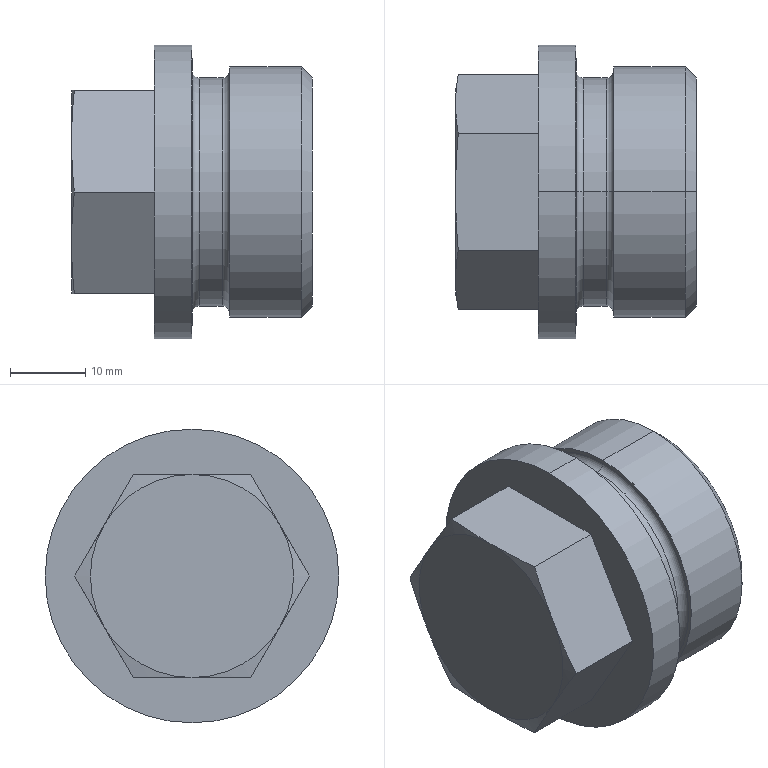Part | SolidWorks | features Boss 1, Cut 1, Fillet 1, Revolution 1 | 1 solid | 29 faces | box 32 x 39 x 39 mm | volume 25996 mm3 | plane 11 | cone 8 | cylinder 6 | torus 4 | commonest cylinder face diameters 30.291 x2 33.249 x2 39 x2
STEP:
#1=CARTESIAN_POINT('',(16.,0.,-16.145));
#2=VERTEX_POINT('',#1);
#3=CARTESIAN_POINT('',(16.,0.,16.145));
#4=VERTEX_POINT('',#3);
#5=CARTESIAN_POINT('',(16.,0.,0.));
#6=DIRECTION('',(-1.,0.,0.));
#7=DIRECTION('',(0.,0.,1.));
#8=AXIS2_PLACEMENT_3D('',#5,#6,#7);
#9=CIRCLE('',#8,16.145);
#10=EDGE_CURVE('',#2,#4,#9,.T.);
#11=ORIENTED_EDGE('',*,*,#10,.F.);
#12=CARTESIAN_POINT('',(17.,0.,-15.145));
#13=VERTEX_POINT('',#12);
#14=CARTESIAN_POINT('',(17.,0.,-16.145));
#15=DIRECTION('',(0.,1.,0.));
#16=DIRECTION('',(0.,0.,1.));
#17=AXIS2_PLACEMENT_3D('',#14,#15,#16);
#18=CIRCLE('',#17,1.);
#19=EDGE_CURVE('',#2,#13,#18,.T.);
#20=ORIENTED_EDGE('',*,*,#19,.T.);
#21=CARTESIAN_POINT('',(17.,0.,15.145));
#22=VERTEX_POINT('',#21);
#23=CARTESIAN_POINT('',(17.,0.,0.));
#24=DIRECTION('',(1.,0.,0.));
#25=DIRECTION('',(0.,0.,1.));
#26=AXIS2_PLACEMENT_3D('',#23,#24,#25);
#27=CIRCLE('',#26,15.145);
#28=EDGE_CURVE('',#22,#13,#27,.T.);
#29=ORIENTED_EDGE('',*,*,#28,.F.);
#30=CARTESIAN_POINT('',(17.,0.,16.145));
#31=DIRECTION('',(0.,-1.,0.));
#32=DIRECTION('',(0.,0.,-1.));
#33=AXIS2_PLACEMENT_3D('',#30,#31,#32);
#34=CIRCLE('',#33,1.);
#35=EDGE_CURVE('',#4,#22,#34,.T.);
#36=ORIENTED_EDGE('',*,*,#35,.F.);
#37=EDGE_LOOP('',(#11,#20,#29,#36));
#38=FACE_OUTER_BOUND('',#37,.T.);
#39=CARTESIAN_POINT('',(17.,0.,0.));
#40=DIRECTION('',(-1.,0.,0.));
#41=DIRECTION('',(0.,0.,1.));
#42=AXIS2_PLACEMENT_3D('',#39,#40,#41);
#43=TOROIDAL_SURFACE('',#42,16.145,1.);
#44=ADVANCED_FACE('',(#38),#43,.F.);
#45=CARTESIAN_POINT('',(21.,0.,16.145));
#46=VERTEX_POINT('',#45);
#47=CARTESIAN_POINT('',(21.,0.,-16.145));
#48=VERTEX_POINT('',#47);
#49=CARTESIAN_POINT('',(21.,0.,0.));
#50=DIRECTION('',(1.,0.,0.));
#51=DIRECTION('',(0.,0.,-1.));
#52=AXIS2_PLACEMENT_3D('',#49,#50,#51);
#53=CIRCLE('',#52,16.145);
#54=EDGE_CURVE('',#46,#48,#53,.T.);
#55=ORIENTED_EDGE('',*,*,#54,.F.);
#56=CARTESIAN_POINT('',(20.,0.,15.145));
#57=VERTEX_POINT('',#56);
#58=CARTESIAN_POINT('',(20.,0.,16.145));
#59=DIRECTION('',(0.,1.,0.));
#60=DIRECTION('',(0.,0.,1.));
#61=AXIS2_PLACEMENT_3D('',#58,#59,#60);
#62=CIRCLE('',#61,1.);
#63=EDGE_CURVE('',#46,#57,#62,.T.);
#64=ORIENTED_EDGE('',*,*,#63,.T.);
#65=CARTESIAN_POINT('',(20.,0.,-15.145));
#66=VERTEX_POINT('',#65);
#67=CARTESIAN_POINT('',(20.,0.,0.));
#68=DIRECTION('',(-1.,0.,0.));
#69=DIRECTION('',(0.,0.,-1.));
#70=AXIS2_PLACEMENT_3D('',#67,#68,#69);
#71=CIRCLE('',#70,15.145);
#72=EDGE_CURVE('',#66,#57,#71,.T.);
#73=ORIENTED_EDGE('',*,*,#72,.F.);
#74=CARTESIAN_POINT('',(20.,0.,-16.145));
#75=DIRECTION('',(0.,-1.,0.));
#76=DIRECTION('',(0.,0.,-1.));
#77=AXIS2_PLACEMENT_3D('',#74,#75,#76);
#78=CIRCLE('',#77,1.);
#79=EDGE_CURVE('',#48,#66,#78,.T.);
#80=ORIENTED_EDGE('',*,*,#79,.F.);
#81=EDGE_LOOP('',(#55,#64,#73,#80));
#82=FACE_OUTER_BOUND('',#81,.T.);
#83=CARTESIAN_POINT('',(20.,0.,0.));
#84=DIRECTION('',(1.,0.,0.));
#85=DIRECTION('',(0.,0.,-1.));
#86=AXIS2_PLACEMENT_3D('',#83,#84,#85);
#87=TOROIDAL_SURFACE('',#86,16.145,1.);
#88=ADVANCED_FACE('',(#82),#87,.F.);
#89=CARTESIAN_POINT('',(32.,0.,15.146));
#90=VERTEX_POINT('',#89);
#91=CARTESIAN_POINT('',(32.,0.,-15.146));
#92=VERTEX_POINT('',#91);
#93=CARTESIAN_POINT('',(32.,0.,0.));
#94=DIRECTION('',(-1.,0.,0.));
#95=DIRECTION('',(0.,0.,1.));
#96=AXIS2_PLACEMENT_3D('',#93,#94,#95);
#97=CIRCLE('',#96,15.146);
#98=EDGE_CURVE('',#90,#92,#97,.T.);
#99=ORIENTED_EDGE('',*,*,#98,.T.);
#100=CARTESIAN_POINT('',(30.521,0.,-16.625));
#101=VERTEX_POINT('',#100);
#102=CARTESIAN_POINT('',(32.,0.,-15.146));
#103=DIRECTION('',(-0.7071,0.,-0.7071));
#104=VECTOR('',#103,1000.);
#105=LINE('',#102,#104);
#106=EDGE_CURVE('',#92,#101,#105,.T.);
#107=ORIENTED_EDGE('',*,*,#106,.T.);
#108=CARTESIAN_POINT('',(30.521,0.,16.625));
#109=VERTEX_POINT('',#108);
#110=CARTESIAN_POINT('',(30.521,0.,0.));
#111=DIRECTION('',(-1.,0.,0.));
#112=DIRECTION('',(0.,0.,1.));
#113=AXIS2_PLACEMENT_3D('',#110,#111,#112);
#114=CIRCLE('',#113,16.625);
#115=EDGE_CURVE('',#109,#101,#114,.T.);
#116=ORIENTED_EDGE('',*,*,#115,.F.);
#117=CARTESIAN_POINT('',(32.,0.,15.146));
#118=DIRECTION('',(-0.7071,0.,0.7071));
#119=VECTOR('',#118,1000.);
#120=LINE('',#117,#119);
#121=EDGE_CURVE('',#90,#109,#120,.T.);
#122=ORIENTED_EDGE('',*,*,#121,.F.);
#123=EDGE_LOOP('',(#99,#107,#116,#122));
#124=FACE_OUTER_BOUND('',#123,.T.);
#125=CARTESIAN_POINT('',(32.,0.,0.));
#126=DIRECTION('',(-1.,0.,0.));
#127=DIRECTION('',(0.,0.,1.));
#128=AXIS2_PLACEMENT_3D('',#125,#126,#127);
#129=CONICAL_SURFACE('',#128,15.146,0.7854);
#130=ADVANCED_FACE('',(#124),#129,.T.);
#131=ORIENTED_EDGE('',*,*,#115,.T.);
#132=CARTESIAN_POINT('',(21.,0.,-16.625));
#133=VERTEX_POINT('',#132);
#134=CARTESIAN_POINT('',(0.,0.,-16.625));
#135=DIRECTION('',(-1.,0.,0.));
#136=VECTOR('',#135,1000.);
#137=LINE('',#134,#136);
#138=EDGE_CURVE('',#101,#133,#137,.T.);
#139=ORIENTED_EDGE('',*,*,#138,.T.);
#140=CARTESIAN_POINT('',(21.,0.,16.625));
#141=VERTEX_POINT('',#140);
#142=CARTESIAN_POINT('',(21.,0.,0.));
#143=DIRECTION('',(-1.,0.,0.));
#144=DIRECTION('',(0.,0.,1.));
#145=AXIS2_PLACEMENT_3D('',#142,#143,#144);
#146=CIRCLE('',#145,16.625);
#147=EDGE_CURVE('',#141,#133,#146,.T.);
#148=ORIENTED_EDGE('',*,*,#147,.F.);
#149=CARTESIAN_POINT('',(0.,0.,16.625));
#150=DIRECTION('',(-1.,0.,0.));
#151=VECTOR('',#150,1000.);
#152=LINE('',#149,#151);
#153=EDGE_CURVE('',#109,#141,#152,.T.);
#154=ORIENTED_EDGE('',*,*,#153,.F.);
#155=EDGE_LOOP('',(#131,#139,#148,#154));
#156=FACE_OUTER_BOUND('',#155,.T.);
#157=CARTESIAN_POINT('',(0.,0.,0.));
#158=DIRECTION('',(-1.,0.,0.));
#159=DIRECTION('',(0.,0.,1.));
#160=AXIS2_PLACEMENT_3D('',#157,#158,#159);
#161=CYLINDRICAL_SURFACE('',#160,16.625);
#162=ADVANCED_FACE('',(#156),#161,.T.);
#163=CARTESIAN_POINT('',(20.,0.,0.));
#164=DIRECTION('',(-1.,0.,0.));
#165=DIRECTION('',(0.,0.,-1.));
#166=AXIS2_PLACEMENT_3D('',#163,#164,#165);
#167=CIRCLE('',#166,15.145);
#168=EDGE_CURVE('',#57,#66,#167,.T.);
#169=ORIENTED_EDGE('',*,*,#168,.T.);
#170=CARTESIAN_POINT('',(0.,0.,-15.145));
#171=DIRECTION('',(-1.,0.,0.));
#172=VECTOR('',#171,1000.);
#173=LINE('',#170,#172);
#174=EDGE_CURVE('',#66,#13,#173,.T.);
#175=ORIENTED_EDGE('',*,*,#174,.T.);
#176=CARTESIAN_POINT('',(17.,0.,0.));
#177=DIRECTION('',(1.,0.,0.));
#178=DIRECTION('',(0.,0.,1.));
#179=AXIS2_PLACEMENT_3D('',#176,#177,#178);
#180=CIRCLE('',#179,15.145);
#181=EDGE_CURVE('',#13,#22,#180,.T.);
#182=ORIENTED_EDGE('',*,*,#181,.T.);
#183=CARTESIAN_POINT('',(0.,0.,15.145));
#184=DIRECTION('',(-1.,0.,0.));
#185=VECTOR('',#184,1000.);
#186=LINE('',#183,#185);
#187=EDGE_CURVE('',#57,#22,#186,.T.);
#188=ORIENTED_EDGE('',*,*,#187,.F.);
#189=EDGE_LOOP('',(#169,#175,#182,#188));
#190=FACE_OUTER_BOUND('',#189,.T.);
#191=CARTESIAN_POINT('',(0.,0.,0.));
#192=DIRECTION('',(-1.,0.,0.));
#193=DIRECTION('',(0.,0.,1.));
#194=AXIS2_PLACEMENT_3D('',#191,#192,#193);
#195=CYLINDRICAL_SURFACE('',#194,15.145);
#196=ADVANCED_FACE('',(#190),#195,.T.);
#197=CARTESIAN_POINT('',(16.,0.,19.5));
#198=VERTEX_POINT('',#197);
#199=CARTESIAN_POINT('',(16.,0.,-19.5));
#200=VERTEX_POINT('',#199);
#201=CARTESIAN_POINT('',(16.,0.,0.));
#202=DIRECTION('',(-1.,0.,0.));
#203=DIRECTION('',(0.,0.,1.));
#204=AXIS2_PLACEMENT_3D('',#201,#202,#203);
#205=CIRCLE('',#204,19.5);
#206=EDGE_CURVE('',#198,#200,#205,.T.);
#207=ORIENTED_EDGE('',*,*,#206,.T.);
#208=CARTESIAN_POINT('',(11.,0.,-19.5));
#209=VERTEX_POINT('',#208);
#210=CARTESIAN_POINT('',(0.,0.,-19.5));
#211=DIRECTION('',(-1.,0.,0.));
#212=VECTOR('',#211,1000.);
#213=LINE('',#210,#212);
#214=EDGE_CURVE('',#200,#209,#213,.T.);
#215=ORIENTED_EDGE('',*,*,#214,.T.);
#216=CARTESIAN_POINT('',(11.,0.,19.5));
#217=VERTEX_POINT('',#216);
#218=CARTESIAN_POINT('',(11.,0.,0.));
#219=DIRECTION('',(-1.,0.,0.));
#220=DIRECTION('',(0.,0.,1.));
#221=AXIS2_PLACEMENT_3D('',#218,#219,#220);
#222=CIRCLE('',#221,19.5);
#223=EDGE_CURVE('',#217,#209,#222,.T.);
#224=ORIENTED_EDGE('',*,*,#223,.F.);
#225=CARTESIAN_POINT('',(0.,0.,19.5));
#226=DIRECTION('',(-1.,0.,0.));
#227=VECTOR('',#226,1000.);
#228=LINE('',#225,#227);
#229=EDGE_CURVE('',#198,#217,#228,.T.);
#230=ORIENTED_EDGE('',*,*,#229,.F.);
#231=EDGE_LOOP('',(#207,#215,#224,#230));
#232=FACE_OUTER_BOUND('',#231,.T.);
#233=CARTESIAN_POINT('',(0.,0.,0.));
#234=DIRECTION('',(-1.,0.,0.));
#235=DIRECTION('',(0.,0.,1.));
#236=AXIS2_PLACEMENT_3D('',#233,#234,#235);
#237=CYLINDRICAL_SURFACE('',#236,19.5);
#238=ADVANCED_FACE('',(#232),#237,.T.);
#239=CARTESIAN_POINT('',(11.,7.794,-13.5));
#240=VERTEX_POINT('',#239);
#241=CARTESIAN_POINT('',(0.3683,7.794,-13.5));
#242=VERTEX_POINT('',#241);
#243=CARTESIAN_POINT('',(52.243,7.794,-13.5));
#244=DIRECTION('',(-1.,0.,0.));
#245=VECTOR('',#244,1000.);
#246=LINE('',#243,#245);
#247=EDGE_CURVE('',#240,#242,#246,.T.);
#248=ORIENTED_EDGE('',*,*,#247,.T.);
#249=CARTESIAN_POINT('',(0.,11.691,-6.75));
#250=VERTEX_POINT('',#249);
#251=CARTESIAN_POINT('',(0.3683,7.794,-13.5));
#252=CARTESIAN_POINT('',(0.2537,8.444,-12.375));
#253=CARTESIAN_POINT('',(0.1607,9.093,-11.25));
#254=CARTESIAN_POINT('',(0.03367,10.392,-9.));
#255=CARTESIAN_POINT('',(0.,11.042,-7.875));
#256=CARTESIAN_POINT('',(0.,11.691,-6.75));
#257=B_SPLINE_CURVE_WITH_KNOTS('',3,(#251,#252,#253,#254,#255,#256),.UNSPECIFIED.,.F.,.F.,(4,2,4),(0.000000231,0.003897,0.007794),.UNSPECIFIED.);
#258=EDGE_CURVE('',#242,#250,#257,.T.);
#259=ORIENTED_EDGE('',*,*,#258,.T.);
#260=CARTESIAN_POINT('',(0.3683,15.588,0.));
#261=VERTEX_POINT('',#260);
#262=CARTESIAN_POINT('',(0.,11.691,-6.75));
#263=CARTESIAN_POINT('',(0.,12.341,-5.625));
#264=CARTESIAN_POINT('',(0.03367,12.99,-4.5));
#265=CARTESIAN_POINT('',(0.1607,14.289,-2.25));
#266=CARTESIAN_POINT('',(0.2537,14.939,-1.125));
#267=CARTESIAN_POINT('',(0.3683,15.588,0.));
#268=B_SPLINE_CURVE_WITH_KNOTS('',3,(#262,#263,#264,#265,#266,#267),.UNSPECIFIED.,.F.,.F.,(4,2,4),(0.007794,0.01169,0.01559),.UNSPECIFIED.);
#269=EDGE_CURVE('',#250,#261,#268,.T.);
#270=ORIENTED_EDGE('',*,*,#269,.T.);
#271=CARTESIAN_POINT('',(11.,15.588,0.));
#272=VERTEX_POINT('',#271);
#273=CARTESIAN_POINT('',(52.243,15.588,0.));
#274=DIRECTION('',(-1.,0.,0.));
#275=VECTOR('',#274,1000.);
#276=LINE('',#273,#275);
#277=EDGE_CURVE('',#272,#261,#276,.T.);
#278=ORIENTED_EDGE('',*,*,#277,.F.);
#279=CARTESIAN_POINT('',(11.,15.588,0.));
#280=DIRECTION('',(0.,-0.5,-0.866));
#281=VECTOR('',#280,1000.);
#282=LINE('',#279,#281);
#283=EDGE_CURVE('',#272,#240,#282,.T.);
#284=ORIENTED_EDGE('',*,*,#283,.T.);
#285=EDGE_LOOP('',(#248,#259,#270,#278,#284));
#286=FACE_OUTER_BOUND('',#285,.T.);
#287=CARTESIAN_POINT('',(52.243,15.588,0.));
#288=DIRECTION('',(0.,0.866,-0.5));
#289=DIRECTION('',(0.,0.5,0.866));
#290=AXIS2_PLACEMENT_3D('',#287,#288,#289);
#291=PLANE('',#290);
#292=ADVANCED_FACE('',(#286),#291,.T.);
#293=CARTESIAN_POINT('',(11.,-7.794,-13.5));
#294=VERTEX_POINT('',#293);
#295=CARTESIAN_POINT('',(0.3683,-7.794,-13.5));
#296=VERTEX_POINT('',#295);
#297=CARTESIAN_POINT('',(52.243,-7.794,-13.5));
#298=DIRECTION('',(-1.,0.,0.));
#299=VECTOR('',#298,1000.);
#300=LINE('',#297,#299);
#301=EDGE_CURVE('',#294,#296,#300,.T.);
#302=ORIENTED_EDGE('',*,*,#301,.T.);
#303=CARTESIAN_POINT('',(0.,0.,-13.5));
#304=VERTEX_POINT('',#303);
#305=CARTESIAN_POINT('',(0.3683,-7.794,-13.5));
#306=CARTESIAN_POINT('',(0.2539,-6.497,-13.5));
#307=CARTESIAN_POINT('',(0.1607,-5.196,-13.5));
#308=CARTESIAN_POINT('',(0.03364,-2.597,-13.5));
#309=CARTESIAN_POINT('',(0.,-1.298,-13.5));
#310=CARTESIAN_POINT('',(0.,0.,-13.5));
#311=B_SPLINE_CURVE_WITH_KNOTS('',3,(#305,#306,#307,#308,#309,#310),.UNSPECIFIED.,.F.,.F.,(4,2,4),(0.01311,0.01702,0.02092),.UNSPECIFIED.);
#312=EDGE_CURVE('',#296,#304,#311,.T.);
#313=ORIENTED_EDGE('',*,*,#312,.T.);
#314=CARTESIAN_POINT('',(0.,0.,-13.5));
#315=CARTESIAN_POINT('',(0.,1.3,-13.5));
#316=CARTESIAN_POINT('',(0.03372,2.6,-13.5));
#317=CARTESIAN_POINT('',(0.1608,5.198,-13.5));
#318=CARTESIAN_POINT('',(0.2538,6.496,-13.5));
#319=CARTESIAN_POINT('',(0.3683,7.794,-13.5));
#320=B_SPLINE_CURVE_WITH_KNOTS('',3,(#314,#315,#316,#317,#318,#319),.UNSPECIFIED.,.F.,.F.,(4,2,4),(0.02092,0.02483,0.02874),.UNSPECIFIED.);
#321=EDGE_CURVE('',#304,#242,#320,.T.);
#322=ORIENTED_EDGE('',*,*,#321,.T.);
#323=ORIENTED_EDGE('',*,*,#247,.F.);
#324=CARTESIAN_POINT('',(11.,7.794,-13.5));
#325=DIRECTION('',(0.,-1.,0.));
#326=VECTOR('',#325,1000.);
#327=LINE('',#324,#326);
#328=EDGE_CURVE('',#240,#294,#327,.T.);
#329=ORIENTED_EDGE('',*,*,#328,.T.);
#330=EDGE_LOOP('',(#302,#313,#322,#323,#329));
#331=FACE_OUTER_BOUND('',#330,.T.);
#332=CARTESIAN_POINT('',(52.243,7.794,-13.5));
#333=DIRECTION('',(0.,0.,-1.));
#334=DIRECTION('',(-1.,0.,0.));
#335=AXIS2_PLACEMENT_3D('',#332,#333,#334);
#336=PLANE('',#335);
#337=ADVANCED_FACE('',(#331),#336,.T.);
#338=CARTESIAN_POINT('',(11.,-15.588,0.));
#339=VERTEX_POINT('',#338);
#340=CARTESIAN_POINT('',(0.3683,-15.588,0.));
#341=VERTEX_POINT('',#340);
#342=CARTESIAN_POINT('',(52.243,-15.588,0.));
#343=DIRECTION('',(-1.,0.,0.));
#344=VECTOR('',#343,1000.);
#345=LINE('',#342,#344);
#346=EDGE_CURVE('',#339,#341,#345,.T.);
#347=ORIENTED_EDGE('',*,*,#346,.T.);
#348=CARTESIAN_POINT('',(0.,-11.691,-6.75));
#349=VERTEX_POINT('',#348);
#350=CARTESIAN_POINT('',(0.3683,-15.588,0.));
#351=CARTESIAN_POINT('',(0.2537,-14.939,-1.125));
#352=CARTESIAN_POINT('',(0.1607,-14.289,-2.25));
#353=CARTESIAN_POINT('',(0.03367,-12.99,-4.5));
#354=CARTESIAN_POINT('',(0.,-12.341,-5.625));
#355=CARTESIAN_POINT('',(0.,-11.691,-6.75));
#356=B_SPLINE_CURVE_WITH_KNOTS('',3,(#350,#351,#352,#353,#354,#355),.UNSPECIFIED.,.F.,.F.,(4,2,4),(0.000000231,0.003897,0.007794),.UNSPECIFIED.);
#357=EDGE_CURVE('',#341,#349,#356,.T.);
#358=ORIENTED_EDGE('',*,*,#357,.T.);
#359=CARTESIAN_POINT('',(0.,-11.691,-6.75));
#360=CARTESIAN_POINT('',(0.,-11.042,-7.875));
#361=CARTESIAN_POINT('',(0.03367,-10.392,-9.));
#362=CARTESIAN_POINT('',(0.1607,-9.093,-11.25));
#363=CARTESIAN_POINT('',(0.2537,-8.444,-12.375));
#364=CARTESIAN_POINT('',(0.3683,-7.794,-13.5));
#365=B_SPLINE_CURVE_WITH_KNOTS('',3,(#359,#360,#361,#362,#363,#364),.UNSPECIFIED.,.F.,.F.,(4,2,4),(0.007794,0.01169,0.01559),.UNSPECIFIED.);
#366=EDGE_CURVE('',#349,#296,#365,.T.);
#367=ORIENTED_EDGE('',*,*,#366,.T.);
#368=ORIENTED_EDGE('',*,*,#301,.F.);
#369=CARTESIAN_POINT('',(11.,-7.794,-13.5));
#370=DIRECTION('',(0.,-0.5,0.866));
#371=VECTOR('',#370,1000.);
#372=LINE('',#369,#371);
#373=EDGE_CURVE('',#294,#339,#372,.T.);
#374=ORIENTED_EDGE('',*,*,#373,.T.);
#375=EDGE_LOOP('',(#347,#358,#367,#368,#374));
#376=FACE_OUTER_BOUND('',#375,.T.);
#377=CARTESIAN_POINT('',(52.243,-7.794,-13.5));
#378=DIRECTION('',(0.,-0.866,-0.5));
#379=DIRECTION('',(0.,0.5,-0.866));
#380=AXIS2_PLACEMENT_3D('',#377,#378,#379);
#381=PLANE('',#380);
#382=ADVANCED_FACE('',(#376),#381,.T.);
#383=CARTESIAN_POINT('',(11.,-7.794,13.5));
#384=VERTEX_POINT('',#383);
#385=CARTESIAN_POINT('',(0.3683,-7.794,13.5));
#386=VERTEX_POINT('',#385);
#387=CARTESIAN_POINT('',(52.243,-7.794,13.5));
#388=DIRECTION('',(-1.,0.,0.));
#389=VECTOR('',#388,1000.);
#390=LINE('',#387,#389);
#391=EDGE_CURVE('',#384,#386,#390,.T.);
#392=ORIENTED_EDGE('',*,*,#391,.T.);
#393=CARTESIAN_POINT('',(0.,-11.691,6.75));
#394=VERTEX_POINT('',#393);
#395=CARTESIAN_POINT('',(0.3683,-7.794,13.5));
#396=CARTESIAN_POINT('',(0.2537,-8.444,12.375));
#397=CARTESIAN_POINT('',(0.1607,-9.093,11.25));
#398=CARTESIAN_POINT('',(0.03367,-10.392,9.));
#399=CARTESIAN_POINT('',(0.,-11.042,7.875));
#400=CARTESIAN_POINT('',(0.,-11.691,6.75));
#401=B_SPLINE_CURVE_WITH_KNOTS('',3,(#395,#396,#397,#398,#399,#400),.UNSPECIFIED.,.F.,.F.,(4,2,4),(0.000000231,0.003897,0.007794),.UNSPECIFIED.);
#402=EDGE_CURVE('',#386,#394,#401,.T.);
#403=ORIENTED_EDGE('',*,*,#402,.T.);
#404=CARTESIAN_POINT('',(0.,-11.691,6.75));
#405=CARTESIAN_POINT('',(0.,-12.341,5.625));
#406=CARTESIAN_POINT('',(0.03367,-12.99,4.5));
#407=CARTESIAN_POINT('',(0.1607,-14.289,2.25));
#408=CARTESIAN_POINT('',(0.2537,-14.939,1.125));
#409=CARTESIAN_POINT('',(0.3683,-15.588,0.));
#410=B_SPLINE_CURVE_WITH_KNOTS('',3,(#404,#405,#406,#407,#408,#409),.UNSPECIFIED.,.F.,.F.,(4,2,4),(0.007794,0.01169,0.01559),.UNSPECIFIED.);
#411=EDGE_CURVE('',#394,#341,#410,.T.);
#412=ORIENTED_EDGE('',*,*,#411,.T.);
#413=ORIENTED_EDGE('',*,*,#346,.F.);
#414=CARTESIAN_POINT('',(11.,-15.588,0.));
#415=DIRECTION('',(0.,0.5,0.866));
#416=VECTOR('',#415,1000.);
#417=LINE('',#414,#416);
#418=EDGE_CURVE('',#339,#384,#417,.T.);
#419=ORIENTED_EDGE('',*,*,#418,.T.);
#420=EDGE_LOOP('',(#392,#403,#412,#413,#419));
#421=FACE_OUTER_BOUND('',#420,.T.);
#422=CARTESIAN_POINT('',(52.243,-15.588,0.));
#423=DIRECTION('',(0.,-0.866,0.5));
#424=DIRECTION('',(0.,-0.5,-0.866));
#425=AXIS2_PLACEMENT_3D('',#422,#423,#424);
#426=PLANE('',#425);
#427=ADVANCED_FACE('',(#421),#426,.T.);
#428=CARTESIAN_POINT('',(11.,7.794,13.5));
#429=VERTEX_POINT('',#428);
#430=CARTESIAN_POINT('',(0.3683,7.794,13.5));
#431=VERTEX_POINT('',#430);
#432=CARTESIAN_POINT('',(52.243,7.794,13.5));
#433=DIRECTION('',(-1.,0.,0.));
#434=VECTOR('',#433,1000.);
#435=LINE('',#432,#434);
#436=EDGE_CURVE('',#429,#431,#435,.T.);
#437=ORIENTED_EDGE('',*,*,#436,.T.);
#438=CARTESIAN_POINT('',(0.,0.,13.5));
#439=VERTEX_POINT('',#438);
#440=CARTESIAN_POINT('',(0.3683,7.794,13.5));
#441=CARTESIAN_POINT('',(0.2538,6.496,13.5));
#442=CARTESIAN_POINT('',(0.1608,5.198,13.5));
#443=CARTESIAN_POINT('',(0.03372,2.6,13.5));
#444=CARTESIAN_POINT('',(0.,1.3,13.5));
#445=CARTESIAN_POINT('',(0.,0.,13.5));
#446=B_SPLINE_CURVE_WITH_KNOTS('',3,(#440,#441,#442,#443,#444,#445),.UNSPECIFIED.,.F.,.F.,(4,2,4),(0.03715,0.04105,0.04496),.UNSPECIFIED.);
#447=EDGE_CURVE('',#431,#439,#446,.T.);
#448=ORIENTED_EDGE('',*,*,#447,.T.);
#449=CARTESIAN_POINT('',(0.,0.,13.5));
#450=CARTESIAN_POINT('',(0.,-1.298,13.5));
#451=CARTESIAN_POINT('',(0.03364,-2.597,13.5));
#452=CARTESIAN_POINT('',(0.1607,-5.196,13.5));
#453=CARTESIAN_POINT('',(0.2539,-6.497,13.5));
#454=CARTESIAN_POINT('',(0.3683,-7.794,13.5));
#455=B_SPLINE_CURVE_WITH_KNOTS('',3,(#449,#450,#451,#452,#453,#454),.UNSPECIFIED.,.F.,.F.,(4,2,4),(0.04496,0.04886,0.05276),.UNSPECIFIED.);
#456=EDGE_CURVE('',#439,#386,#455,.T.);
#457=ORIENTED_EDGE('',*,*,#456,.T.);
#458=ORIENTED_EDGE('',*,*,#391,.F.);
#459=CARTESIAN_POINT('',(11.,-7.794,13.5));
#460=DIRECTION('',(0.,1.,0.));
#461=VECTOR('',#460,1000.);
#462=LINE('',#459,#461);
#463=EDGE_CURVE('',#384,#429,#462,.T.);
#464=ORIENTED_EDGE('',*,*,#463,.T.);
#465=EDGE_LOOP('',(#437,#448,#457,#458,#464));
#466=FACE_OUTER_BOUND('',#465,.T.);
#467=CARTESIAN_POINT('',(52.243,-7.794,13.5));
#468=DIRECTION('',(0.,0.,1.));
#469=DIRECTION('',(0.,-1.,0.));
#470=AXIS2_PLACEMENT_3D('',#467,#468,#469);
#471=PLANE('',#470);
#472=ADVANCED_FACE('',(#466),#471,.T.);
#473=ORIENTED_EDGE('',*,*,#277,.T.);
#474=CARTESIAN_POINT('',(0.,11.691,6.75));
#475=VERTEX_POINT('',#474);
#476=CARTESIAN_POINT('',(0.3683,15.588,0.));
#477=CARTESIAN_POINT('',(0.2537,14.939,1.125));
#478=CARTESIAN_POINT('',(0.1607,14.289,2.25));
#479=CARTESIAN_POINT('',(0.03367,12.99,4.5));
#480=CARTESIAN_POINT('',(0.,12.341,5.625));
#481=CARTESIAN_POINT('',(0.,11.691,6.75));
#482=B_SPLINE_CURVE_WITH_KNOTS('',3,(#476,#477,#478,#479,#480,#481),.UNSPECIFIED.,.F.,.F.,(4,2,4),(0.000000231,0.003897,0.007794),.UNSPECIFIED.);
#483=EDGE_CURVE('',#261,#475,#482,.T.);
#484=ORIENTED_EDGE('',*,*,#483,.T.);
#485=CARTESIAN_POINT('',(0.,11.691,6.75));
#486=CARTESIAN_POINT('',(0.,11.042,7.875));
#487=CARTESIAN_POINT('',(0.03367,10.392,9.));
#488=CARTESIAN_POINT('',(0.1607,9.093,11.25));
#489=CARTESIAN_POINT('',(0.2537,8.444,12.375));
#490=CARTESIAN_POINT('',(0.3683,7.794,13.5));
#491=B_SPLINE_CURVE_WITH_KNOTS('',3,(#485,#486,#487,#488,#489,#490),.UNSPECIFIED.,.F.,.F.,(4,2,4),(0.007794,0.01169,0.01559),.UNSPECIFIED.);
#492=EDGE_CURVE('',#475,#431,#491,.T.);
#493=ORIENTED_EDGE('',*,*,#492,.T.);
#494=ORIENTED_EDGE('',*,*,#436,.F.);
#495=CARTESIAN_POINT('',(11.,7.794,13.5));
#496=DIRECTION('',(0.,0.5,-0.866));
#497=VECTOR('',#496,1000.);
#498=LINE('',#495,#497);
#499=EDGE_CURVE('',#429,#272,#498,.T.);
#500=ORIENTED_EDGE('',*,*,#499,.T.);
#501=EDGE_LOOP('',(#473,#484,#493,#494,#500));
#502=FACE_OUTER_BOUND('',#501,.T.);
#503=CARTESIAN_POINT('',(52.243,7.794,13.5));
#504=DIRECTION('',(0.,0.866,0.5));
#505=DIRECTION('',(0.,-0.5,0.866));
#506=AXIS2_PLACEMENT_3D('',#503,#504,#505);
#507=PLANE('',#506);
#508=ADVANCED_FACE('',(#502),#507,.T.);
#509=ORIENTED_EDGE('',*,*,#328,.F.);
#510=ORIENTED_EDGE('',*,*,#283,.F.);
#511=ORIENTED_EDGE('',*,*,#499,.F.);
#512=ORIENTED_EDGE('',*,*,#463,.F.);
#513=ORIENTED_EDGE('',*,*,#418,.F.);
#514=ORIENTED_EDGE('',*,*,#373,.F.);
#515=EDGE_LOOP('',(#509,#510,#511,#512,#513,#514));
#516=FACE_BOUND('',#515,.T.);
#517=ORIENTED_EDGE('',*,*,#223,.T.);
#518=CARTESIAN_POINT('',(11.,0.,0.));
#519=DIRECTION('',(-1.,0.,0.));
#520=DIRECTION('',(0.,0.,1.));
#521=AXIS2_PLACEMENT_3D('',#518,#519,#520);
#522=CIRCLE('',#521,19.5);
#523=EDGE_CURVE('',#209,#217,#522,.T.);
#524=ORIENTED_EDGE('',*,*,#523,.T.);
#525=EDGE_LOOP('',(#517,#524));
#526=FACE_OUTER_BOUND('',#525,.T.);
#527=CARTESIAN_POINT('',(11.,19.5,0.));
#528=DIRECTION('',(1.,0.,0.));
#529=DIRECTION('',(0.,0.,-1.));
#530=AXIS2_PLACEMENT_3D('',#527,#528,#529);
#531=PLANE('',#530);
#532=ADVANCED_FACE('',(#516,#526),#531,.F.);
#533=ORIENTED_EDGE('',*,*,#214,.F.);
#534=CARTESIAN_POINT('',(16.,0.,0.));
#535=DIRECTION('',(-1.,0.,0.));
#536=DIRECTION('',(0.,0.,1.));
#537=AXIS2_PLACEMENT_3D('',#534,#535,#536);
#538=CIRCLE('',#537,19.5);
#539=EDGE_CURVE('',#200,#198,#538,.T.);
#540=ORIENTED_EDGE('',*,*,#539,.T.);
#541=ORIENTED_EDGE('',*,*,#229,.T.);
#542=ORIENTED_EDGE('',*,*,#523,.F.);
#543=EDGE_LOOP('',(#533,#540,#541,#542));
#544=FACE_OUTER_BOUND('',#543,.T.);
#545=CARTESIAN_POINT('',(0.,0.,0.));
#546=DIRECTION('',(-1.,0.,0.));
#547=DIRECTION('',(0.,0.,1.));
#548=AXIS2_PLACEMENT_3D('',#545,#546,#547);
#549=CYLINDRICAL_SURFACE('',#548,19.5);
#550=ADVANCED_FACE('',(#544),#549,.T.);
#551=CARTESIAN_POINT('',(16.,0.,0.));
#552=DIRECTION('',(-1.,0.,0.));
#553=DIRECTION('',(0.,0.,1.));
#554=AXIS2_PLACEMENT_3D('',#551,#552,#553);
#555=CIRCLE('',#554,16.145);
#556=EDGE_CURVE('',#4,#2,#555,.T.);
#557=ORIENTED_EDGE('',*,*,#556,.T.);
#558=ORIENTED_EDGE('',*,*,#10,.T.);
#559=EDGE_LOOP('',(#557,#558));
#560=FACE_BOUND('',#559,.T.);
#561=ORIENTED_EDGE('',*,*,#206,.F.);
#562=ORIENTED_EDGE('',*,*,#539,.F.);
#563=EDGE_LOOP('',(#561,#562));
#564=FACE_OUTER_BOUND('',#563,.T.);
#565=CARTESIAN_POINT('',(16.,15.145,0.));
#566=DIRECTION('',(-1.,0.,0.));
#567=DIRECTION('',(0.,0.,1.));
#568=AXIS2_PLACEMENT_3D('',#565,#566,#567);
#569=PLANE('',#568);
#570=ADVANCED_FACE('',(#560,#564),#569,.F.);
#571=ORIENTED_EDGE('',*,*,#174,.F.);
#572=ORIENTED_EDGE('',*,*,#72,.T.);
#573=ORIENTED_EDGE('',*,*,#187,.T.);
#574=ORIENTED_EDGE('',*,*,#28,.T.);
#575=EDGE_LOOP('',(#571,#572,#573,#574));
#576=FACE_OUTER_BOUND('',#575,.T.);
#577=CARTESIAN_POINT('',(0.,0.,0.));
#578=DIRECTION('',(-1.,0.,0.));
#579=DIRECTION('',(0.,0.,1.));
#580=AXIS2_PLACEMENT_3D('',#577,#578,#579);
#581=CYLINDRICAL_SURFACE('',#580,15.145);
#582=ADVANCED_FACE('',(#576),#581,.T.);
#583=CARTESIAN_POINT('',(21.,0.,0.));
#584=DIRECTION('',(1.,0.,0.));
#585=DIRECTION('',(0.,0.,-1.));
#586=AXIS2_PLACEMENT_3D('',#583,#584,#585);
#587=CIRCLE('',#586,16.145);
#588=EDGE_CURVE('',#48,#46,#587,.T.);
#589=ORIENTED_EDGE('',*,*,#588,.T.);
#590=ORIENTED_EDGE('',*,*,#54,.T.);
#591=EDGE_LOOP('',(#589,#590));
#592=FACE_BOUND('',#591,.T.);
#593=ORIENTED_EDGE('',*,*,#147,.T.);
#594=CARTESIAN_POINT('',(21.,0.,0.));
#595=DIRECTION('',(-1.,0.,0.));
#596=DIRECTION('',(0.,0.,1.));
#597=AXIS2_PLACEMENT_3D('',#594,#595,#596);
#598=CIRCLE('',#597,16.625);
#599=EDGE_CURVE('',#133,#141,#598,.T.);
#600=ORIENTED_EDGE('',*,*,#599,.T.);
#601=EDGE_LOOP('',(#593,#600));
#602=FACE_OUTER_BOUND('',#601,.T.);
#603=CARTESIAN_POINT('',(21.,16.625,0.));
#604=DIRECTION('',(1.,0.,0.));
#605=DIRECTION('',(0.,0.,-1.));
#606=AXIS2_PLACEMENT_3D('',#603,#604,#605);
#607=PLANE('',#606);
#608=ADVANCED_FACE('',(#592,#602),#607,.F.);
#609=ORIENTED_EDGE('',*,*,#138,.F.);
#610=CARTESIAN_POINT('',(30.521,0.,0.));
#611=DIRECTION('',(-1.,0.,0.));
#612=DIRECTION('',(0.,0.,1.));
#613=AXIS2_PLACEMENT_3D('',#610,#611,#612);
#614=CIRCLE('',#613,16.625);
#615=EDGE_CURVE('',#101,#109,#614,.T.);
#616=ORIENTED_EDGE('',*,*,#615,.T.);
#617=ORIENTED_EDGE('',*,*,#153,.T.);
#618=ORIENTED_EDGE('',*,*,#599,.F.);
#619=EDGE_LOOP('',(#609,#616,#617,#618));
#620=FACE_OUTER_BOUND('',#619,.T.);
#621=CARTESIAN_POINT('',(0.,0.,0.));
#622=DIRECTION('',(-1.,0.,0.));
#623=DIRECTION('',(0.,0.,1.));
#624=AXIS2_PLACEMENT_3D('',#621,#622,#623);
#625=CYLINDRICAL_SURFACE('',#624,16.625);
#626=ADVANCED_FACE('',(#620),#625,.T.);
#627=ORIENTED_EDGE('',*,*,#106,.F.);
#628=CARTESIAN_POINT('',(32.,0.,0.));
#629=DIRECTION('',(-1.,0.,0.));
#630=DIRECTION('',(0.,0.,1.));
#631=AXIS2_PLACEMENT_3D('',#628,#629,#630);
#632=CIRCLE('',#631,15.146);
#633=EDGE_CURVE('',#92,#90,#632,.T.);
#634=ORIENTED_EDGE('',*,*,#633,.T.);
#635=ORIENTED_EDGE('',*,*,#121,.T.);
#636=ORIENTED_EDGE('',*,*,#615,.F.);
#637=EDGE_LOOP('',(#627,#634,#635,#636));
#638=FACE_OUTER_BOUND('',#637,.T.);
#639=CARTESIAN_POINT('',(32.,0.,0.));
#640=DIRECTION('',(-1.,0.,0.));
#641=DIRECTION('',(0.,0.,1.));
#642=AXIS2_PLACEMENT_3D('',#639,#640,#641);
#643=CONICAL_SURFACE('',#642,15.146,0.7854);
#644=ADVANCED_FACE('',(#638),#643,.T.);
#645=ORIENTED_EDGE('',*,*,#98,.F.);
#646=ORIENTED_EDGE('',*,*,#633,.F.);
#647=EDGE_LOOP('',(#645,#646));
#648=FACE_OUTER_BOUND('',#647,.T.);
#649=CARTESIAN_POINT('',(32.,15.146,0.));
#650=DIRECTION('',(-1.,0.,0.));
#651=DIRECTION('',(0.,0.,1.));
#652=AXIS2_PLACEMENT_3D('',#649,#650,#651);
#653=PLANE('',#652);
#654=ADVANCED_FACE('',(#648),#653,.F.);
#655=CARTESIAN_POINT('',(0.,0.,0.));
#656=DIRECTION('',(1.,0.,0.));
#657=DIRECTION('',(0.,0.,-1.));
#658=AXIS2_PLACEMENT_3D('',#655,#656,#657);
#659=CIRCLE('',#658,13.5);
#660=EDGE_CURVE('',#349,#304,#659,.T.);
#661=ORIENTED_EDGE('',*,*,#660,.T.);
#662=ORIENTED_EDGE('',*,*,#312,.F.);
#663=ORIENTED_EDGE('',*,*,#366,.F.);
#664=EDGE_LOOP('',(#661,#662,#663));
#665=FACE_OUTER_BOUND('',#664,.T.);
#666=CARTESIAN_POINT('',(0.,0.,0.));
#667=DIRECTION('',(1.,0.,0.));
#668=DIRECTION('',(0.,0.,1.));
#669=AXIS2_PLACEMENT_3D('',#666,#667,#668);
#670=CONICAL_SURFACE('',#669,13.5,1.396);
#671=ADVANCED_FACE('',(#665),#670,.T.);
#672=ORIENTED_EDGE('',*,*,#411,.F.);
#673=CARTESIAN_POINT('',(0.,0.,0.));
#674=DIRECTION('',(1.,0.,0.));
#675=DIRECTION('',(0.,0.,-1.));
#676=AXIS2_PLACEMENT_3D('',#673,#674,#675);
#677=CIRCLE('',#676,13.5);
#678=EDGE_CURVE('',#394,#349,#677,.T.);
#679=ORIENTED_EDGE('',*,*,#678,.T.);
#680=ORIENTED_EDGE('',*,*,#357,.F.);
#681=EDGE_LOOP('',(#672,#679,#680));
#682=FACE_OUTER_BOUND('',#681,.T.);
#683=CARTESIAN_POINT('',(0.,0.,0.));
#684=DIRECTION('',(1.,0.,0.));
#685=DIRECTION('',(0.,0.,1.));
#686=AXIS2_PLACEMENT_3D('',#683,#684,#685);
#687=CONICAL_SURFACE('',#686,13.5,1.396);
#688=ADVANCED_FACE('',(#682),#687,.T.);
#689=ORIENTED_EDGE('',*,*,#456,.F.);
#690=CARTESIAN_POINT('',(0.,0.,0.));
#691=DIRECTION('',(1.,0.,0.));
#692=DIRECTION('',(0.,0.,-1.));
#693=AXIS2_PLACEMENT_3D('',#690,#691,#692);
#694=CIRCLE('',#693,13.5);
#695=EDGE_CURVE('',#439,#394,#694,.T.);
#696=ORIENTED_EDGE('',*,*,#695,.T.);
#697=ORIENTED_EDGE('',*,*,#402,.F.);
#698=EDGE_LOOP('',(#689,#696,#697));
#699=FACE_OUTER_BOUND('',#698,.T.);
#700=CARTESIAN_POINT('',(0.,0.,0.));
#701=DIRECTION('',(1.,0.,0.));
#702=DIRECTION('',(0.,0.,1.));
#703=AXIS2_PLACEMENT_3D('',#700,#701,#702);
#704=CONICAL_SURFACE('',#703,13.5,1.396);
#705=ADVANCED_FACE('',(#699),#704,.T.);
#706=ORIENTED_EDGE('',*,*,#492,.F.);
#707=CARTESIAN_POINT('',(0.,0.,0.));
#708=DIRECTION('',(-1.,0.,0.));
#709=DIRECTION('',(0.,0.,1.));
#710=AXIS2_PLACEMENT_3D('',#707,#708,#709);
#711=CIRCLE('',#710,13.5);
#712=EDGE_CURVE('',#439,#475,#711,.T.);
#713=ORIENTED_EDGE('',*,*,#712,.F.);
#714=ORIENTED_EDGE('',*,*,#447,.F.);
#715=EDGE_LOOP('',(#706,#713,#714));
#716=FACE_OUTER_BOUND('',#715,.T.);
#717=CARTESIAN_POINT('',(0.,0.,0.));
#718=DIRECTION('',(1.,0.,0.));
#719=DIRECTION('',(0.,0.,1.));
#720=AXIS2_PLACEMENT_3D('',#717,#718,#719);
#721=CONICAL_SURFACE('',#720,13.5,1.396);
#722=ADVANCED_FACE('',(#716),#721,.T.);
#723=CARTESIAN_POINT('',(0.,0.,0.));
#724=DIRECTION('',(1.,0.,0.));
#725=DIRECTION('',(0.,0.,-1.));
#726=AXIS2_PLACEMENT_3D('',#723,#724,#725);
#727=CIRCLE('',#726,13.5);
#728=EDGE_CURVE('',#250,#475,#727,.T.);
#729=ORIENTED_EDGE('',*,*,#728,.T.);
#730=ORIENTED_EDGE('',*,*,#483,.F.);
#731=ORIENTED_EDGE('',*,*,#269,.F.);
#732=EDGE_LOOP('',(#729,#730,#731));
#733=FACE_OUTER_BOUND('',#732,.T.);
#734=CARTESIAN_POINT('',(0.,0.,0.));
#735=DIRECTION('',(1.,0.,0.));
#736=DIRECTION('',(0.,0.,1.));
#737=AXIS2_PLACEMENT_3D('',#734,#735,#736);
#738=CONICAL_SURFACE('',#737,13.5,1.396);
#739=ADVANCED_FACE('',(#733),#738,.T.);
#740=CARTESIAN_POINT('',(0.,0.,0.));
#741=DIRECTION('',(1.,0.,0.));
#742=DIRECTION('',(0.,0.,-1.));
#743=AXIS2_PLACEMENT_3D('',#740,#741,#742);
#744=CIRCLE('',#743,13.5);
#745=EDGE_CURVE('',#304,#250,#744,.T.);
#746=ORIENTED_EDGE('',*,*,#745,.T.);
#747=ORIENTED_EDGE('',*,*,#258,.F.);
#748=ORIENTED_EDGE('',*,*,#321,.F.);
#749=EDGE_LOOP('',(#746,#747,#748));
#750=FACE_OUTER_BOUND('',#749,.T.);
#751=CARTESIAN_POINT('',(0.,0.,0.));
#752=DIRECTION('',(1.,0.,0.));
#753=DIRECTION('',(0.,0.,1.));
#754=AXIS2_PLACEMENT_3D('',#751,#752,#753);
#755=CONICAL_SURFACE('',#754,13.5,1.396);
#756=ADVANCED_FACE('',(#750),#755,.T.);
#757=ORIENTED_EDGE('',*,*,#745,.F.);
#758=ORIENTED_EDGE('',*,*,#660,.F.);
#759=ORIENTED_EDGE('',*,*,#678,.F.);
#760=ORIENTED_EDGE('',*,*,#695,.F.);
#761=ORIENTED_EDGE('',*,*,#712,.T.);
#762=ORIENTED_EDGE('',*,*,#728,.F.);
#763=EDGE_LOOP('',(#757,#758,#759,#760,#761,#762));
#764=FACE_OUTER_BOUND('',#763,.T.);
#765=CARTESIAN_POINT('',(0.,1.5,0.));
#766=DIRECTION('',(1.,0.,0.));
#767=DIRECTION('',(0.,0.,-1.));
#768=AXIS2_PLACEMENT_3D('',#765,#766,#767);
#769=PLANE('',#768);
#770=ADVANCED_FACE('',(#764),#769,.F.);
#771=ORIENTED_EDGE('',*,*,#63,.F.);
#772=ORIENTED_EDGE('',*,*,#588,.F.);
#773=ORIENTED_EDGE('',*,*,#79,.T.);
#774=ORIENTED_EDGE('',*,*,#168,.F.);
#775=EDGE_LOOP('',(#771,#772,#773,#774));
#776=FACE_OUTER_BOUND('',#775,.T.);
#777=CARTESIAN_POINT('',(20.,0.,0.));
#778=DIRECTION('',(1.,0.,0.));
#779=DIRECTION('',(0.,0.,-1.));
#780=AXIS2_PLACEMENT_3D('',#777,#778,#779);
#781=TOROIDAL_SURFACE('',#780,16.145,1.);
#782=ADVANCED_FACE('',(#776),#781,.F.);
#783=ORIENTED_EDGE('',*,*,#19,.F.);
#784=ORIENTED_EDGE('',*,*,#556,.F.);
#785=ORIENTED_EDGE('',*,*,#35,.T.);
#786=ORIENTED_EDGE('',*,*,#181,.F.);
#787=EDGE_LOOP('',(#783,#784,#785,#786));
#788=FACE_OUTER_BOUND('',#787,.T.);
#789=CARTESIAN_POINT('',(17.,0.,0.));
#790=DIRECTION('',(-1.,0.,0.));
#791=DIRECTION('',(0.,0.,1.));
#792=AXIS2_PLACEMENT_3D('',#789,#790,#791);
#793=TOROIDAL_SURFACE('',#792,16.145,1.);
#794=ADVANCED_FACE('',(#788),#793,.F.);
#795=CLOSED_SHELL('',(#44,#88,#130,#162,#196,#238,#292,#337,#382,#427,#472,#508,#532,#550,#570,#582,#608,#626,#644,#654,#671,#688,#705,#722,#739,#756,#770,#782,#794));
#796=MANIFOLD_SOLID_BREP('',#795);
#797=CARTESIAN_POINT('',(0.,0.,0.));
#798=DIRECTION('',(0.,0.,1.));
#799=DIRECTION('',(1.,0.,0.));
#800=AXIS2_PLACEMENT_3D('',#797,#798,#799);
#801=(LENGTH_UNIT()NAMED_UNIT(*)SI_UNIT(.MILLI.,.METRE.));
#802=UNCERTAINTY_MEASURE_WITH_UNIT(LENGTH_MEASURE(0.00001),#801,'','');
#803=(NAMED_UNIT(*)PLANE_ANGLE_UNIT()SI_UNIT($,.RADIAN.));
#804=(NAMED_UNIT(*)SI_UNIT($,.STERADIAN.)SOLID_ANGLE_UNIT());
#805=(GEOMETRIC_REPRESENTATION_CONTEXT(3)GLOBAL_UNCERTAINTY_ASSIGNED_CONTEXT((#802))GLOBAL_UNIT_ASSIGNED_CONTEXT((#801,#803,#804))REPRESENTATION_CONTEXT('',''));
#806=ADVANCED_BREP_SHAPE_REPRESENTATION('',(#796,#800),#805);